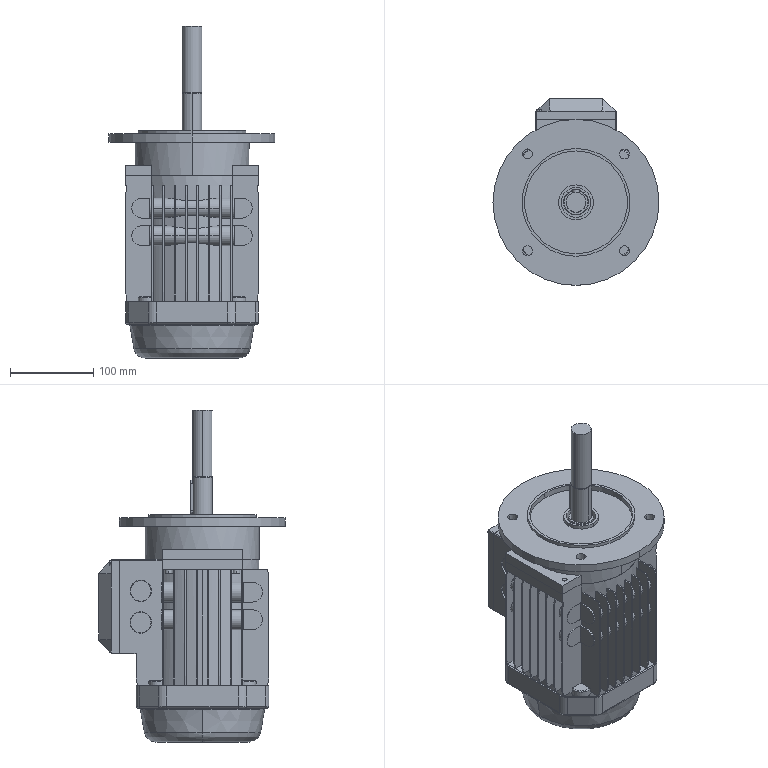Part | SolidWorks | features ICE 39, Fillet 15, MirrorPattern 11, Extrusion 5, Revolution 5, CirPattern 4, LibraryFeature 3, Chamfer 2, Dome 2, LPattern 2, CombineBodies 1, Shell 1 | 3 solids | 1272 faces | box 200 x 225.2 x 400 mm | volume 5238989 mm3 | plane 1023 | cylinder 189 | torus 44 | cone 14 | sphere 2 | commonest cylinder face diameters 24 x58 6 x20 137.6 x20 2 x16 10 x14 4 x12